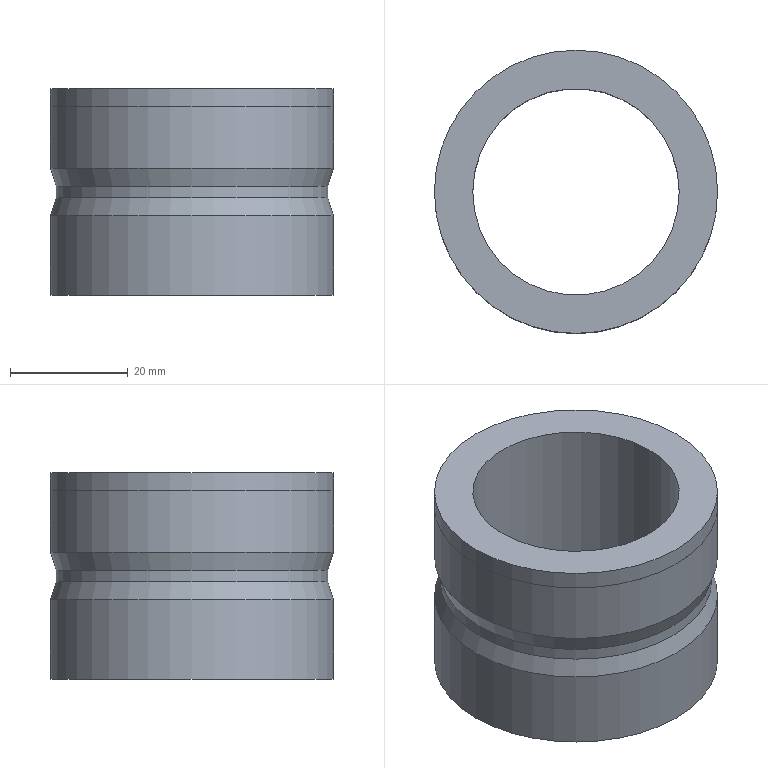Part | STEP file | 1_id458_xmt_txt | 1 solid | 10 faces | box 48.005 x 48.005 x 35 mm | volume 28920 mm3 | cylinder 5 | plane 3 | cone 2 | commonest cylinder face diameters 48 x2 35 x1 46 x1 48.005 x1
STEP:
#1=CARTESIAN_POINT('',(-186.,302.,114.5));
#2=VERTEX_POINT('',#1);
#3=CARTESIAN_POINT('',(-162.,302.,114.5));
#4=DIRECTION('',(0.,0.,-1.));
#5=DIRECTION('',(-1.,0.,0.));
#6=AXIS2_PLACEMENT_3D('',#3,#4,#5);
#7=CIRCLE('',#6,24.);
#8=EDGE_CURVE('',#2,#2,#7,.T.);
#9=ORIENTED_EDGE('',*,*,#8,.T.);
#10=EDGE_LOOP('',(#9));
#11=FACE_BOUND('',#10,.T.);
#12=CARTESIAN_POINT('',(-186.,302.,101.));
#13=VERTEX_POINT('',#12);
#14=CARTESIAN_POINT('',(-162.,302.,101.));
#15=DIRECTION('',(0.,0.,-1.));
#16=DIRECTION('',(-1.,0.,0.));
#17=AXIS2_PLACEMENT_3D('',#14,#15,#16);
#18=CIRCLE('',#17,24.);
#19=EDGE_CURVE('',#13,#13,#18,.T.);
#20=ORIENTED_EDGE('',*,*,#19,.F.);
#21=EDGE_LOOP('',(#20));
#22=FACE_BOUND('',#21,.T.);
#23=CARTESIAN_POINT('',(-162.,302.,118.5));
#24=DIRECTION('',(0.,0.,-1.));
#25=DIRECTION('',(1.,0.,0.));
#26=AXIS2_PLACEMENT_3D('',#23,#24,#25);
#27=CYLINDRICAL_SURFACE('',#26,24.);
#28=ADVANCED_FACE('',(#11,#22),#27,.T.);
#29=CARTESIAN_POINT('',(-186.002,302.,136.));
#30=VERTEX_POINT('',#29);
#31=CARTESIAN_POINT('',(-162.,302.,136.));
#32=DIRECTION('',(0.,0.,1.));
#33=DIRECTION('',(-1.,0.,0.));
#34=AXIS2_PLACEMENT_3D('',#31,#32,#33);
#35=CIRCLE('',#34,24.003);
#36=EDGE_CURVE('',#30,#30,#35,.T.);
#37=ORIENTED_EDGE('',*,*,#36,.F.);
#38=EDGE_LOOP('',(#37));
#39=FACE_BOUND('',#38,.T.);
#40=CARTESIAN_POINT('',(-186.002,302.,133.));
#41=VERTEX_POINT('',#40);
#42=CARTESIAN_POINT('',(-162.,302.,133.));
#43=DIRECTION('',(0.,0.,-1.));
#44=DIRECTION('',(-1.,0.,0.));
#45=AXIS2_PLACEMENT_3D('',#42,#43,#44);
#46=CIRCLE('',#45,24.003);
#47=EDGE_CURVE('',#41,#41,#46,.T.);
#48=ORIENTED_EDGE('',*,*,#47,.F.);
#49=EDGE_LOOP('',(#48));
#50=FACE_BOUND('',#49,.T.);
#51=CARTESIAN_POINT('',(-162.,302.,134.5));
#52=DIRECTION('',(0.,0.,-1.));
#53=DIRECTION('',(1.,0.,0.));
#54=AXIS2_PLACEMENT_3D('',#51,#52,#53);
#55=CYLINDRICAL_SURFACE('',#54,24.003);
#56=ADVANCED_FACE('',(#39,#50),#55,.T.);
#57=CARTESIAN_POINT('',(-179.5,302.,101.));
#58=VERTEX_POINT('',#57);
#59=CARTESIAN_POINT('',(-162.,302.,101.));
#60=DIRECTION('',(0.,0.,1.));
#61=DIRECTION('',(-1.,0.,0.));
#62=AXIS2_PLACEMENT_3D('',#59,#60,#61);
#63=CIRCLE('',#62,17.5);
#64=EDGE_CURVE('',#58,#58,#63,.T.);
#65=ORIENTED_EDGE('',*,*,#64,.F.);
#66=EDGE_LOOP('',(#65));
#67=FACE_BOUND('',#66,.T.);
#68=CARTESIAN_POINT('',(-179.5,302.,136.));
#69=VERTEX_POINT('',#68);
#70=CARTESIAN_POINT('',(-162.,302.,136.));
#71=DIRECTION('',(0.,0.,-1.));
#72=DIRECTION('',(-1.,0.,0.));
#73=AXIS2_PLACEMENT_3D('',#70,#71,#72);
#74=CIRCLE('',#73,17.5);
#75=EDGE_CURVE('',#69,#69,#74,.T.);
#76=ORIENTED_EDGE('',*,*,#75,.F.);
#77=EDGE_LOOP('',(#76));
#78=FACE_BOUND('',#77,.T.);
#79=CARTESIAN_POINT('',(-162.,302.,118.5));
#80=DIRECTION('',(0.,0.,-1.));
#81=DIRECTION('',(1.,0.,0.));
#82=AXIS2_PLACEMENT_3D('',#79,#80,#81);
#83=CYLINDRICAL_SURFACE('',#82,17.5);
#84=ADVANCED_FACE('',(#67,#78),#83,.F.);
#85=CARTESIAN_POINT('',(-186.,302.,133.));
#86=VERTEX_POINT('',#85);
#87=CARTESIAN_POINT('',(-162.,302.,133.));
#88=DIRECTION('',(0.,0.,-1.));
#89=DIRECTION('',(-1.,0.,0.));
#90=AXIS2_PLACEMENT_3D('',#87,#88,#89);
#91=CIRCLE('',#90,24.);
#92=EDGE_CURVE('',#86,#86,#91,.T.);
#93=ORIENTED_EDGE('',*,*,#92,.T.);
#94=EDGE_LOOP('',(#93));
#95=FACE_BOUND('',#94,.T.);
#96=CARTESIAN_POINT('',(-186.,302.,122.5));
#97=VERTEX_POINT('',#96);
#98=CARTESIAN_POINT('',(-162.,302.,122.5));
#99=DIRECTION('',(0.,0.,1.));
#100=DIRECTION('',(-1.,0.,0.));
#101=AXIS2_PLACEMENT_3D('',#98,#99,#100);
#102=CIRCLE('',#101,24.);
#103=EDGE_CURVE('',#97,#97,#102,.T.);
#104=ORIENTED_EDGE('',*,*,#103,.T.);
#105=EDGE_LOOP('',(#104));
#106=FACE_BOUND('',#105,.T.);
#107=CARTESIAN_POINT('',(-162.,302.,118.5));
#108=DIRECTION('',(0.,0.,-1.));
#109=DIRECTION('',(1.,0.,0.));
#110=AXIS2_PLACEMENT_3D('',#107,#108,#109);
#111=CYLINDRICAL_SURFACE('',#110,24.);
#112=ADVANCED_FACE('',(#95,#106),#111,.T.);
#113=CARTESIAN_POINT('',(-139.,302.,119.5));
#114=VERTEX_POINT('',#113);
#115=CARTESIAN_POINT('',(-162.,302.,119.5));
#116=DIRECTION('',(0.,0.,-1.));
#117=DIRECTION('',(1.,0.,0.));
#118=AXIS2_PLACEMENT_3D('',#115,#116,#117);
#119=CIRCLE('',#118,23.);
#120=EDGE_CURVE('',#114,#114,#119,.T.);
#121=ORIENTED_EDGE('',*,*,#120,.F.);
#122=EDGE_LOOP('',(#121));
#123=FACE_BOUND('',#122,.T.);
#124=ORIENTED_EDGE('',*,*,#103,.F.);
#125=EDGE_LOOP('',(#124));
#126=FACE_BOUND('',#125,.T.);
#127=CARTESIAN_POINT('',(-162.,302.,121.));
#128=DIRECTION('',(0.,0.,1.));
#129=DIRECTION('',(-1.,0.,0.));
#130=AXIS2_PLACEMENT_3D('',#127,#128,#129);
#131=CONICAL_SURFACE('',#130,23.5,18.435);
#132=ADVANCED_FACE('',(#123,#126),#131,.T.);
#133=CARTESIAN_POINT('',(-139.,302.,117.5));
#134=VERTEX_POINT('',#133);
#135=CARTESIAN_POINT('',(-162.,302.,117.5));
#136=DIRECTION('',(0.,0.,-1.));
#137=DIRECTION('',(1.,0.,0.));
#138=AXIS2_PLACEMENT_3D('',#135,#136,#137);
#139=CIRCLE('',#138,23.);
#140=EDGE_CURVE('',#134,#134,#139,.T.);
#141=ORIENTED_EDGE('',*,*,#140,.F.);
#142=EDGE_LOOP('',(#141));
#143=FACE_BOUND('',#142,.T.);
#144=ORIENTED_EDGE('',*,*,#120,.T.);
#145=EDGE_LOOP('',(#144));
#146=FACE_BOUND('',#145,.T.);
#147=CARTESIAN_POINT('',(-162.,302.,118.5));
#148=DIRECTION('',(0.,0.,-1.));
#149=DIRECTION('',(-1.,0.,0.));
#150=AXIS2_PLACEMENT_3D('',#147,#148,#149);
#151=CYLINDRICAL_SURFACE('',#150,23.);
#152=ADVANCED_FACE('',(#143,#146),#151,.T.);
#153=ORIENTED_EDGE('',*,*,#8,.F.);
#154=EDGE_LOOP('',(#153));
#155=FACE_BOUND('',#154,.T.);
#156=ORIENTED_EDGE('',*,*,#140,.T.);
#157=EDGE_LOOP('',(#156));
#158=FACE_BOUND('',#157,.T.);
#159=CARTESIAN_POINT('',(-162.,302.,116.));
#160=DIRECTION('',(0.,0.,-1.));
#161=DIRECTION('',(-1.,0.,0.));
#162=AXIS2_PLACEMENT_3D('',#159,#160,#161);
#163=CONICAL_SURFACE('',#162,23.5,18.435);
#164=ADVANCED_FACE('',(#155,#158),#163,.T.);
#165=ORIENTED_EDGE('',*,*,#47,.T.);
#166=EDGE_LOOP('',(#165));
#167=FACE_BOUND('',#166,.T.);
#168=ORIENTED_EDGE('',*,*,#92,.F.);
#169=EDGE_LOOP('',(#168));
#170=FACE_BOUND('',#169,.T.);
#171=CARTESIAN_POINT('',(-162.,302.,133.));
#172=DIRECTION('',(0.,0.,-1.));
#173=DIRECTION('',(1.,0.,0.));
#174=AXIS2_PLACEMENT_3D('',#171,#172,#173);
#175=PLANE('',#174);
#176=ADVANCED_FACE('',(#167,#170),#175,.T.);
#177=ORIENTED_EDGE('',*,*,#75,.T.);
#178=EDGE_LOOP('',(#177));
#179=FACE_BOUND('',#178,.T.);
#180=ORIENTED_EDGE('',*,*,#36,.T.);
#181=EDGE_LOOP('',(#180));
#182=FACE_BOUND('',#181,.T.);
#183=CARTESIAN_POINT('',(-162.,302.,136.));
#184=DIRECTION('',(0.,0.,1.));
#185=DIRECTION('',(-1.,0.,0.));
#186=AXIS2_PLACEMENT_3D('',#183,#184,#185);
#187=PLANE('',#186);
#188=ADVANCED_FACE('',(#179,#182),#187,.T.);
#189=ORIENTED_EDGE('',*,*,#64,.T.);
#190=EDGE_LOOP('',(#189));
#191=FACE_BOUND('',#190,.T.);
#192=ORIENTED_EDGE('',*,*,#19,.T.);
#193=EDGE_LOOP('',(#192));
#194=FACE_BOUND('',#193,.T.);
#195=CARTESIAN_POINT('',(-162.,302.,101.));
#196=DIRECTION('',(0.,0.,-1.));
#197=DIRECTION('',(1.,0.,0.));
#198=AXIS2_PLACEMENT_3D('',#195,#196,#197);
#199=PLANE('',#198);
#200=ADVANCED_FACE('',(#191,#194),#199,.T.);
#201=CLOSED_SHELL('',(#28,#56,#84,#112,#132,#152,#164,#176,#188,#200));
#202=MANIFOLD_SOLID_BREP('',#201);
#203=(LENGTH_UNIT()NAMED_UNIT(*)SI_UNIT(.MILLI.,.METRE.));
#204=UNCERTAINTY_MEASURE_WITH_UNIT(LENGTH_MEASURE(0.00002),#203,'','');
#205=(NAMED_UNIT(*)PLANE_ANGLE_UNIT()SI_UNIT($,.RADIAN.));
#206=PLANE_ANGLE_MEASURE_WITH_UNIT(PLANE_ANGLE_MEASURE(0.01745),#205);
#207=DIMENSIONAL_EXPONENTS(0.,0.,0.,0.,0.,0.,0.);
#208=(CONVERSION_BASED_UNIT('DEGREE',#206)NAMED_UNIT(#207)PLANE_ANGLE_UNIT());
#209=(NAMED_UNIT(*)SI_UNIT($,.STERADIAN.)SOLID_ANGLE_UNIT());
#210=(GEOMETRIC_REPRESENTATION_CONTEXT(3)GLOBAL_UNCERTAINTY_ASSIGNED_CONTEXT((#204))GLOBAL_UNIT_ASSIGNED_CONTEXT((#203,#208,#209))REPRESENTATION_CONTEXT('',''));
#211=ADVANCED_BREP_SHAPE_REPRESENTATION('',(#202),#210);